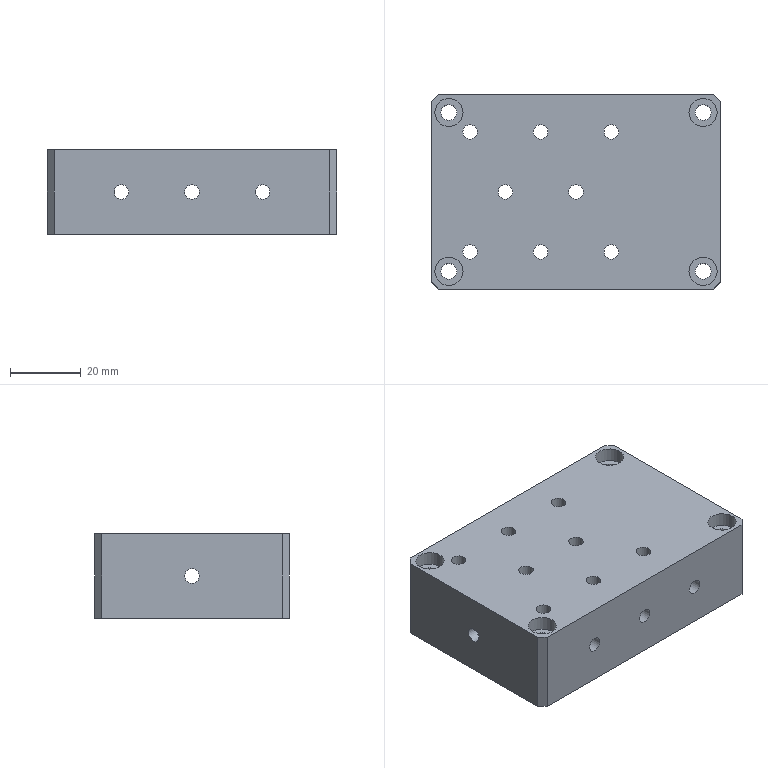NC program | NX | posted with a generic post | part box 82 x 55 x 24 mm
Whole program:
N10 G17 G21 G94 G90
(FLOOR_WALL_COPY , TOOL : D80)
N12 T19 M6
N14 G54
N16 G17 G0 G90 X-84. Y0. B0. C0. S6500 M3
N18 G43 Z30. H19
N20 Z8.
N22 G94 G1 Z5. F1500.
N24 X-81.
N26 X81.
N28 X84.
N30 Z8.
N32 G0 Z30.
N34 X-84.
N36 Z7.
N38 G1 Z4.
N40 X-81.
N42 X81.
N44 X84.
N46 Z7.
N48 G0 Z30.
N50 X-84.
N52 Z6.
N54 G1 Z3.
N56 X-81.
N58 X81.
N60 X84.
N62 Z6.
N64 G0 Z30.
N66 X-84.
N68 Z5.
N70 G1 Z2.
N72 X-81.
N74 X81.
N76 X84.
N78 Z5.
N80 G0 Z30.
N82 X-84.
N84 Z4.
N86 G1 Z1.
N88 X-81.
N90 X81.
N92 X84.
N94 Z4.
N96 G0 Z30.
N98 X-84.
N100 Z3.
N102 G1 Z0.
N104 X-81.
N106 X81.
N108 X84.
N110 Z3.
N112 G0 Z30.
N114 M5
(FLOOR_WALL_1 , TOOL : D10)
N116 T15 M6
N118 G54
N120 G17 G0 G90 X1.172 Y-4.308 B0. C0. S9500 M3
N122 G43 Z30. H15
N124 Z1.
N126 G94 G3 X1.172 Y-4.308 Z0.177 I-1.172 J2.208 F1000.
N128 X1.172 Y-4.308 Z-0.646 I-1.172 J2.208
N130 X0. Y0.4 Z-0.994 R2.5
N132 G1 X-13.9 F3500.
N134 Y-0.4
N136 X13.9
N138 Y0.4
N140 X0.
N142 Y7.9
N144 X-21.4
N146 Y-7.9
N148 X21.4
N150 Y7.9
N152 X0.
N154 Y15.4
N156 X-28.
N158 G3 X-28.9 Y14.5 R0.9
N160 G1 Y-14.5
N162 G3 X-28. Y-15.4 R0.9
N164 G1 X28.
N166 G3 X28.9 Y-14.5 R0.9
N168 G1 Y14.5
N170 G3 X28. Y15.4 R0.9
N172 G1 X0.
N174 Z0.006
N176 G0 X1.172 Y-4.308
N178 G3 X1.172 Y-4.308 Z-0.817 I-1.172 J2.208 F1000.
N180 X1.172 Y-4.308 Z-1.641 I-1.172 J2.208
N182 X0. Y0.4 Z-1.988 R2.5
N184 G1 X-13.9 F3500.
N186 Y-0.4
N188 X13.9
N190 Y0.4
N192 X0.
N194 Y7.9
N196 X-21.4
N198 Y-7.9
N200 X21.4
N202 Y7.9
N204 X0.
N206 Y15.4
N208 X-28.
N210 G3 X-28.9 Y14.5 R0.9
N212 G1 Y-14.5
N214 G3 X-28. Y-15.4 R0.9
N216 G1 X28.
N218 G3 X28.9 Y-14.5 R0.9
N220 G1 Y14.5
N222 G3 X28. Y15.4 R0.9
N224 G1 X0.
N226 Z-0.988
N228 G0 X1.172 Y-4.308
N230 G3 X1.172 Y-4.308 Z-1.811 I-1.172 J2.208 F1000.
N232 X1.172 Y-4.308 Z-2.635 I-1.172 J2.208
N234 X0. Y0.4 Z-2.982 R2.5
N236 G1 X-13.9 F3500.
N238 Y-0.4
N240 X13.9
N242 Y0.4
N244 X0.
N246 Y7.9
N248 X-21.4
N250 Y-7.9
N252 X21.4
N254 Y7.9
N256 X0.
N258 Y15.4
N260 X-28.
N262 G3 X-28.9 Y14.5 R0.9
N264 G1 Y-14.5
N266 G3 X-28. Y-15.4 R0.9
N268 G1 X28.
N270 G3 X28.9 Y-14.5 R0.9
N272 G1 Y14.5
N274 G3 X28. Y15.4 R0.9
N276 G1 X0.
N278 Z-1.982
N280 G0 X1.172 Y-4.308
N282 G3 X1.172 Y-4.308 Z-2.806 I-1.172 J2.208 F1000.
N284 X1.172 Y-4.308 Z-3.629 I-1.172 J2.208
N286 X0. Y0.4 Z-3.976 R2.5
N288 G1 X-13.9 F3500.
N290 Y-0.4
N292 X13.9
N294 Y0.4
N296 X0.
N298 Y7.9
N300 X-21.4
N302 Y-7.9
N304 X21.4
N306 Y7.9
N308 X0.
N310 Y15.4
N312 X-28.
N314 G3 X-28.9 Y14.5 R0.9
N316 G1 Y-14.5
N318 G3 X-28. Y-15.4 R0.9
N320 G1 X28.
N322 G3 X28.9 Y-14.5 R0.9
N324 G1 Y14.5
N326 G3 X28. Y15.4 R0.9
N328 G1 X0.
N330 Z-2.976
N332 G0 X1.172 Y-4.308
N334 G3 X1.172 Y-4.308 Z-3.8 I-1.172 J2.208 F1000.
N336 X1.172 Y-4.308 Z-4.623 I-1.172 J2.208
N338 X0. Y0.4 Z-4.971 R2.5
N340 G1 X-13.9 F3500.
N342 Y-0.4
N344 X13.9
N346 Y0.4
N348 X0.
N350 Y7.9
N352 X-21.4
N354 Y-7.9
N356 X21.4
N358 Y7.9
N360 X0.
N362 Y15.4
N364 X-28.
N366 G3 X-28.9 Y14.5 R0.9
N368 G1 Y-14.5
N370 G3 X-28. Y-15.4 R0.9
N372 G1 X28.
N374 G3 X28.9 Y-14.5 R0.9
N376 G1 Y14.5
N378 G3 X28. Y15.4 R0.9
N380 G1 X0.
N382 Z-3.971
N384 G0 X1.172 Y-4.308
N386 G3 X1.172 Y-4.308 Z-4.794 I-1.172 J2.208 F1000.
N388 X1.172 Y-4.308 Z-5.617 I-1.172 J2.208
N390 X0. Y0.4 Z-5.965 R2.5
N392 G1 X-13.9 F3500.
N394 Y-0.4
N396 X13.9
N398 Y0.4
N400 X0.
N402 Y7.9
N404 X-21.4
N406 Y-7.9
N408 X21.4
N410 Y7.9
N412 X0.
N414 Y15.4
N416 X-28.
N418 G3 X-28.9 Y14.5 R0.9
N420 G1 Y-14.5
N422 G3 X-28. Y-15.4 R0.9
N424 G1 X28.
N426 G3 X28.9 Y-14.5 R0.9
N428 G1 Y14.5
N430 G3 X28. Y15.4 R0.9
N432 G1 X0.
N434 Z-4.965
N436 G0 X1.172 Y-4.308
N438 G3 X1.172 Y-4.308 Z-5.788 I-1.172 J2.208 F1000.
N440 X1.172 Y-4.308 Z-6.611 I-1.172 J2.208
N442 X0. Y0.4 Z-6.959 R2.5
N444 G1 X-13.9 F3500.
N446 Y-0.4
N448 X13.9
N450 Y0.4
N452 X0.
N454 Y7.9
N456 X-21.4
N458 Y-7.9
N460 X21.4
N462 Y7.9
N464 X0.
N466 Y15.4
N468 X-28.
N470 G3 X-28.9 Y14.5 R0.9
N472 G1 Y-14.5
N474 G3 X-28. Y-15.4 R0.9
N476 G1 X28.
N478 G3 X28.9 Y-14.5 R0.9
N480 G1 Y14.5
N482 G3 X28. Y15.4 R0.9
N484 G1 X0.
N486 Z-5.959
N488 G0 X1.172 Y-4.308
N490 G3 X1.172 Y-4.308 Z-6.782 I-1.172 J2.208 F1000.
N492 X1.172 Y-4.308 Z-7.605 I-1.172 J2.208
N494 X0. Y0.4 Z-7.953 R2.5
N496 G1 X-13.9 F3500.
N498 Y-0.4
N500 X13.9
N502 Y0.4
N504 X0.
N506 Y7.9
N508 X-21.4
N510 Y-7.9
N512 X21.4
N514 Y7.9
N516 X0.
N518 Y15.4
N520 X-28.
N522 G3 X-28.9 Y14.5 R0.9
N524 G1 Y-14.5
N526 G3 X-28. Y-15.4 R0.9
N528 G1 X28.
N530 G3 X28.9 Y-14.5 R0.9
N532 G1 Y14.5
N534 G3 X28. Y15.4 R0.9
N536 G1 X0.
N538 Z-6.953
N540 G0 X1.172 Y-4.308
N542 G3 X1.172 Y-4.308 Z-7.776 I-1.172 J2.208 F1000.
N544 X1.172 Y-4.308 Z-8.599 I-1.172 J2.208
N546 X0. Y0.4 Z-8.947 R2.5
N548 G1 X-13.9 F3500.
N550 Y-0.4
N552 X13.9
N554 Y0.4
N556 X0.
N558 Y7.9
N560 X-21.4
N562 Y-7.9
N564 X21.4
N566 Y7.9
N568 X0.
N570 Y15.4
N572 X-28.
N574 G3 X-28.9 Y14.5 R0.9
N576 G1 Y-14.5
N578 G3 X-28. Y-15.4 R0.9
N580 G1 X28.
N582 G3 X28.9 Y-14.5 R0.9
N584 G1 Y14.5
N586 G3 X28. Y15.4 R0.9
N588 G1 X0.
N590 Z-7.947
N592 G0 X1.172 Y-4.308
N594 G3 X1.172 Y-4.308 Z-8.77 I-1.172 J2.208 F1000.
N596 X1.172 Y-4.308 Z-9.593 I-1.172 J2.208
N598 X0. Y0.4 Z-9.941 R2.5
N600 G1 X-13.9 F3500.
N602 Y-0.4
N604 X13.9
N606 Y0.4
N608 X0.
N610 Y7.9
N612 X-21.4
N614 Y-7.9
N616 X21.4
N618 Y7.9
N620 X0.
N622 Y15.4
N624 X-28.
N626 G3 X-28.9 Y14.5 R0.9
N628 G1 Y-14.5
N630 G3 X-28. Y-15.4 R0.9
N632 G1 X28.
N634 G3 X28.9 Y-14.5 R0.9
N636 G1 Y14.5
N638 G3 X28. Y15.4 R0.9
N640 G1 X0.
N642 Z-8.941
N644 G0 X1.172 Y-4.308
N646 G3 X1.172 Y-4.308 Z-9.764 I-1.172 J2.208 F1000.
N648 X1.172 Y-4.308 Z-10.588 I-1.172 J2.208
N650 X0. Y0.4 Z-10.935 R2.5
N652 G1 X-13.9 F3500.
N654 Y-0.4
N656 X13.9
N658 Y0.4
N660 X0.
N662 Y7.9
N664 X-21.4
N666 Y-7.9
N668 X21.4
N670 Y7.9
N672 X0.
N674 Y15.4
N676 X-28.
N678 G3 X-28.9 Y14.5 R0.9
N680 G1 Y-14.5
N682 G3 X-28. Y-15.4 R0.9
N684 G1 X28.
N686 G3 X28.9 Y-14.5 R0.9
N688 G1 Y14.5
N690 G3 X28. Y15.4 R0.9
N692 G1 X0.
N694 Z-9.935
N696 G0 X1.172 Y-4.308
N698 G3 X1.172 Y-4.308 Z-10.759 I-1.172 J2.208 F1000.
N700 X1.172 Y-4.308 Z-11.582 I-1.172 J2.208
N702 X0. Y0.4 Z-11.929 R2.5
N704 G1 X-13.9 F3500.
N706 Y-0.4
N708 X13.9
N710 Y0.4
N712 X0.
N714 Y7.9
N716 X-21.4
N718 Y-7.9
N720 X21.4
N722 Y7.9
N724 X0.
N726 Y15.4
N728 X-28.
N730 G3 X-28.9 Y14.5 R0.9
N732 G1 Y-14.5
N734 G3 X-28. Y-15.4 R0.9
N736 G1 X28.
N738 G3 X28.9 Y-14.5 R0.9
N740 G1 Y14.5
N742 G3 X28. Y15.4 R0.9
N744 G1 X0.
N746 Z-10.929
N748 G0 X1.172 Y-4.308
N750 G3 X1.172 Y-4.308 Z-11.753 I-1.172 J2.208 F1000.
N752 X1.172 Y-4.308 Z-12.576 I-1.172 J2.208
N754 X0. Y0.4 Z-12.924 R2.5
N756 G1 X-13.9 F3500.
N758 Y-0.4
N760 X13.9
N762 Y0.4
N764 X0.
N766 Y7.9
N768 X-21.4
N770 Y-7.9
N772 X21.4
N774 Y7.9
N776 X0.
N778 Y15.4
N780 X-28.
N782 G3 X-28.9 Y14.5 R0.9
N784 G1 Y-14.5
N786 G3 X-28. Y-15.4 R0.9
N788 G1 X28.
N790 G3 X28.9 Y-14.5 R0.9
N792 G1 Y14.5
N794 G3 X28. Y15.4 R0.9
N796 G1 X0.
N798 Z-11.924
N800 G0 X1.172 Y-4.308
N802 G3 X1.172 Y-4.308 Z-12.747 I-1.172 J2.208 F1000.
N804 X1.172 Y-4.308 Z-13.57 I-1.172 J2.208
N806 X0. Y0.4 Z-13.918 R2.5
N808 G1 X-13.9 F3500.
N810 Y-0.4
N812 X13.9
N814 Y0.4
N816 X0.
N818 Y7.9
N820 X-21.4
N822 Y-7.9
N824 X21.4
N826 Y7.9
N828 X0.
N830 Y15.4
N832 X-28.
N834 G3 X-28.9 Y14.5 R0.9
N836 G1 Y-14.5
N838 G3 X-28. Y-15.4 R0.9
N840 G1 X28.
N842 G3 X28.9 Y-14.5 R0.9
N844 G1 Y14.5
N846 G3 X28. Y15.4 R0.9
N848 G1 X0.
N850 Z-12.918
N852 G0 X1.172 Y-4.308
N854 G3 X1.172 Y-4.308 Z-13.741 I-1.172 J2.208 F1000.
N856 X1.172 Y-4.308 Z-14.564 I-1.172 J2.208
N858 X0. Y0.4 Z-14.912 R2.5
N860 G1 X-13.9 F3500.
N862 Y-0.4
N864 X13.9
N866 Y0.4
N868 X0.
N870 Y7.9
N872 X-21.4
N874 Y-7.9
N876 X21.4
N878 Y7.9
N880 X0.
N882 Y15.4
N884 X-28.
N886 G3 X-28.9 Y14.5 R0.9
N888 G1 Y-14.5
N890 G3 X-28. Y-15.4 R0.9
N892 G1 X28.
N894 G3 X28.9 Y-14.5 R0.9
N896 G1 Y14.5
N898 G3 X28. Y15.4 R0.9
N900 G1 X0.
N902 Z-13.912
N904 G0 X1.172 Y-4.308
N906 G3 X1.172 Y-4.308 Z-14.735 I-1.172 J2.208 F1000.
N908 X1.172 Y-4.308 Z-15.558 I-1.172 J2.208
N910 X0. Y0.4 Z-15.906 R2.5
N912 G1 X-13.9 F3500.
N914 Y-0.4
N916 X13.9
N918 Y0.4
N920 X0.
N922 Y7.9
N924 X-21.4
N926 Y-7.9
N928 X21.4
N930 Y7.9
N932 X0.
N934 Y15.4
N936 X-28.
N938 G3 X-28.9 Y14.5 R0.9
N940 G1 Y-14.5
N942 G3 X-28. Y-15.4 R0.9
N944 G1 X28.
N946 G3 X28.9 Y-14.5 R0.9
N948 G1 Y14.5
N950 G3 X28. Y15.4 R0.9
N952 G1 X0.
N954 Z-14.906
N956 G0 X1.172 Y-4.308
N958 G3 X1.172 Y-4.308 Z-15.729 I-1.172 J2.208 F1000.
N960 X1.172 Y-4.308 Z-16.552 I-1.172 J2.208
N962 X0. Y0.4 Z-16.9 R2.5
N964 G1 X-13.9 F3500.
N966 Y-0.4
N968 X13.9
N970 Y0.4
N972 X0.
N974 Y7.9
N976 X-21.4
N978 Y-7.9
N980 X21.4
N982 Y7.9
N984 X0.
N986 Y15.4
N988 X-28.
N990 G3 X-28.9 Y14.5 R0.9
N992 G1 Y-14.5
N994 G3 X-28. Y-15.4 R0.9
N996 G1 X28.
N998 G3 X28.9 Y-14.5 R0.9
N1000 G1 Y14.5
N1002 G3 X28. Y15.4 R0.9
N1004 G1 X0.
N1006 Z-15.9
N1008 G0 Z30.
(FLOOR_WALL_1_COPY , TOOL : D10)
N1010 Y3.
N1012 Z-14.
N1014 G1 Z-17. F1000.
N1016 Y0.
N1018 X13.5 F1500.
N1020 X-13.5
N1022 X0.
N1024 Y-5.
N1026 X18.5
N1028 Y5.
N1030 X-18.5
N1032 Y-5.
N1034 X0.
N1036 Y-10.
N1038 X23.5
N1040 Y10.
N1042 X-23.5
N1044 Y-10.
N1046 X0.
N1048 Y-15.
N1050 X28.
N1052 G3 X28.5 Y-14.5 R0.5
N1054 G1 Y14.5
N1056 G3 X28. Y15. R0.5
N1058 G1 X-28.
N1060 G3 X-28.5 Y14.5 R0.5
N1062 G1 Y-14.5
N1064 G3 X-28. Y-15. R0.5
N1066 G1 X0.
N1068 Y-12.
N1070 Y-15.5 F1000.
N1072 X28. F1500.
N1074 G3 X29. Y-14.5 R1.
N1076 G1 Y14.5
N1078 G3 X28. Y15.5 R1.
N1080 G1 X-28.
N1082 G3 X-29. Y14.5 R1.
N1084 G1 Y-14.5
N1086 G3 X-28. Y-15.5 R1.
N1088 G1 X0.
N1090 Y-12.5
N1092 Z-14.
N1094 G0 Z30.
N1096 M5
(PLANAR_PROFILE , TOOL : D1.5)
N1098 T16 M6
N1100 G54
N1102 G17 G0 G90 X0. Y-22.05 B0. C0. S9500 M3
N1104 G43 Z30. H16
N1106 Z3.1
N1108 G94 G1 Z0. F850.
N1110 X28. F1150.
N1112 G3 X35.55 Y-14.5 R7.55
N1114 G1 Y14.5
N1116 G3 X28. Y22.05 R7.55
N1118 G1 X-28.
N1120 G3 X-35.55 Y14.5 R7.55
N1122 G1 Y-14.5
N1124 G3 X-28. Y-22.05 R7.55
N1126 G1 X0.
N1128 Z3.
N1130 Z-0.1 F850.
N1132 X28. F1150.
N1134 G3 X35.55 Y-14.5 R7.55
N1136 G1 Y14.5
N1138 G3 X28. Y22.05 R7.55
N1140 G1 X-28.
N1142 G3 X-35.55 Y14.5 R7.55
N1144 G1 Y-14.5
N1146 G3 X-28. Y-22.05 R7.55
N1148 G1 X0.
N1150 Z2.9
N1152 Z-0.2 F850.
N1154 X28. F1150.
N1156 G3 X35.55 Y-14.5 R7.55
N1158 G1 Y14.5
N1160 G3 X28. Y22.05 R7.55
N1162 G1 X-28.
N1164 G3 X-35.55 Y14.5 R7.55
N1166 G1 Y-14.5
N1168 G3 X-28. Y-22.05 R7.55
N1170 G1 X0.
N1172 Z2.8
N1174 Z-0.3 F850.
N1176 X28. F1150.
N1178 G3 X35.55 Y-14.5 R7.55
N1180 G1 Y14.5
N1182 G3 X28. Y22.05 R7.55
N1184 G1 X-28.
N1186 G3 X-35.55 Y14.5 R7.55
N1188 G1 Y-14.5
N1190 G3 X-28. Y-22.05 R7.55
N1192 G1 X0.
N1194 Z2.7
N1196 Z-0.4 F850.
N1198 X28. F1150.
N1200 G3 X35.55 Y-14.5 R7.55
N1202 G1 Y14.5
N1204 G3 X28. Y22.05 R7.55
N1206 G1 X-28.
N1208 G3 X-35.55 Y14.5 R7.55
N1210 G1 Y-14.5
N1212 G3 X-28. Y-22.05 R7.55
N1214 G1 X0.
N1216 Z2.6
N1218 Z-0.5 F850.
N1220 X28. F1150.
N1222 G3 X35.55 Y-14.5 R7.55
N1224 G1 Y14.5
N1226 G3 X28. Y22.05 R7.55
N1228 G1 X-28.
N1230 G3 X-35.55 Y14.5 R7.55
N1232 G1 Y-14.5
N1234 G3 X-28. Y-22.05 R7.55
N1236 G1 X0.
N1238 Z2.5
N1240 Z-0.6 F850.
N1242 X28. F1150.
N1244 G3 X35.55 Y-14.5 R7.55
N1246 G1 Y14.5
N1248 G3 X28. Y22.05 R7.55
N1250 G1 X-28.
N1252 G3 X-35.55 Y14.5 R7.55
N1254 G1 Y-14.5
N1256 G3 X-28. Y-22.05 R7.55
N1258 G1 X0.
N1260 Z2.4
N1262 Z-0.7 F850.
N1264 X28. F1150.
N1266 G3 X35.55 Y-14.5 R7.55
N1268 G1 Y14.5
N1270 G3 X28. Y22.05 R7.55
N1272 G1 X-28.
N1274 G3 X-35.55 Y14.5 R7.55
N1276 G1 Y-14.5
N1278 G3 X-28. Y-22.05 R7.55
N1280 G1 X0.
N1282 Z2.3
N1284 Z-0.8 F850.
N1286 X28. F1150.
N1288 G3 X35.55 Y-14.5 R7.55
N1290 G1 Y14.5
N1292 G3 X28. Y22.05 R7.55
N1294 G1 X-28.
N1296 G3 X-35.55 Y14.5 R7.55
N1298 G1 Y-14.5
N1300 G3 X-28. Y-22.05 R7.55
N1302 G1 X0.
N1304 Z2.2
N1306 Z-0.9 F850.
N1308 X28. F1150.
N1310 G3 X35.55 Y-14.5 R7.55
N1312 G1 Y14.5
N1314 G3 X28. Y22.05 R7.55
N1316 G1 X-28.
N1318 G3 X-35.55 Y14.5 R7.55
N1320 G1 Y-14.5
N1322 G3 X-28. Y-22.05 R7.55
N1324 G1 X0.
N1326 Z2.1
N1328 Z-1. F850.
N1330 X28. F1150.
N1332 G3 X35.55 Y-14.5 R7.55
N1334 G1 Y14.5
N1336 G3 X28. Y22.05 R7.55
N1338 G1 X-28.
N1340 G3 X-35.55 Y14.5 R7.55
N1342 G1 Y-14.5
N1344 G3 X-28. Y-22.05 R7.55
N1346 G1 X0.
N1348 Z2.
N1350 G0 Z30.
N1352 M5
(PLANAR_MILL_COPY_COPY_COPY_COPY , TOOL : D6A45)
N1354 T01 M6
N1356 G54
N1358 G17 G0 G90 X-37.25 Y-21.634 B0. C0. S9500 M3
N1360 G43 Z30. H1
N1362 Z0.9
N1364 G94 G1 Z-0.6 F1250.
N1366 G3 X-37.75 Y-22.5 R1.
N1368 X-36. Y-24.25 R1.75
N1370 X-37.75 Y-22.5 R-1.75
N1372 X-37.25 Y-23.366 R1.
N1374 G1 Z0.9
N1376 G0 Z30.
N1378 Y23.366
N1380 Z0.9
N1382 G1 Z-0.6
N1384 G3 X-37.75 Y22.5 R1.
N1386 X-36. Y20.75 R1.75
N1388 X-37.75 Y22.5 R-1.75
N1390 X-37.25 Y21.634 R1.
N1392 G1 Z0.9
N1394 G0 Z30.
N1396 X-0.866 Y28.5
N1398 Z0.9
N1400 G1 Z-0.6
N1402 G3 X0. Y28. R1.
N1404 G1 X39.
N1406 G2 X39.354 Y27.854 R0.5
N1408 G1 X41.354 Y25.854
N1410 G2 X41.5 Y25.5 R0.5
N1412 G1 Y-25.5
N1414 G2 X41.354 Y-25.854 R0.5
N1416 G1 X39.354 Y-27.854
N1418 G2 X39. Y-28. R0.5
N1420 G1 X-39.
N1422 G2 X-39.354 Y-27.854 R0.5
N1424 G1 X-41.354 Y-25.854
N1426 G2 X-41.5 Y-25.5 R0.5
N1428 G1 Y25.5
N1430 G2 X-41.354 Y25.854 R0.5
N1432 G1 X-39.354 Y27.854
N1434 G2 X-39. Y28. R0.5
N1436 G1 X0.
N1438 G3 X0.866 Y28.5 R1.
N1440 G1 Z0.9
N1442 G0 Z30.
N1444 Y19.5
N1446 Z0.9
N1448 G1 Z-0.6
N1450 G3 X0. Y20. R1.
N1452 G1 X-28.
N1454 G3 X-33.5 Y14.5 R5.5
N1456 G1 Y-14.5
N1458 G3 X-28. Y-20. R5.5
N1460 G1 X28.
N1462 G3 X33.5 Y-14.5 R5.5
N1464 G1 Y14.5
N1466 G3 X28. Y20. R5.5
N1468 G1 X0.
N1470 G3 X-0.866 Y19.5 R1.
N1472 G1 Z0.9
N1474 G0 Z30.
N1476 Y22.3
N1478 Z0.9
N1480 G1 Z-0.6
N1482 G3 X0. Y21.8 R1.
N1484 G1 X28.
N1486 G2 X35.3 Y14.5 R7.3
N1488 G1 Y-14.5
N1490 G2 X28. Y-21.8 R7.3
N1492 G1 X-28.
N1494 G2 X-35.3 Y-14.5 R7.3
N1496 G1 Y14.5
N1498 G2 X-28. Y21.8 R7.3
N1500 G1 X0.
N1502 G3 X0.866 Y22.3 R1.
N1504 G1 Z0.9
N1506 G0 Z30.
N1508 Y21.8
N1510 Z0.9
N1512 G1 Z-0.6
N1514 G3 X0. Y22.3 R1.
N1516 G1 X-28.
N1518 G3 X-35.8 Y14.5 R7.8
N1520 G1 Y-14.5
N1522 G3 X-28. Y-22.3 R7.8
N1524 G1 X28.
N1526 G3 X35.8 Y-14.5 R7.8
N1528 G1 Y14.5
N1530 G3 X28. Y22.3 R7.8
N1532 G1 X0.
N1534 G3 X-0.866 Y21.8 R1.
N1536 G1 Z0.9
N1538 G0 Z30.
N1540 X36.866 Y23.75
N1542 Z0.9
N1544 G1 Z-0.6
N1546 G3 X36. Y24.25 R1.
N1548 X34.25 Y22.5 R1.75
N1550 X36. Y24.25 R-1.75
N1552 X35.134 Y23.75 R1.
N1554 G1 Z0.9
N1556 G0 Z30.
N1558 X37.25 Y-23.366
N1560 Z0.9
N1562 G1 Z-0.6
N1564 G3 X37.75 Y-22.5 R1.
N1566 X36. Y-20.75 R1.75
N1568 X37.75 Y-22.5 R-1.75
N1570 X37.25 Y-21.634 R1.
N1572 G1 Z0.9
N1574 G0 Z30.
N1576 M5
N1578 M2